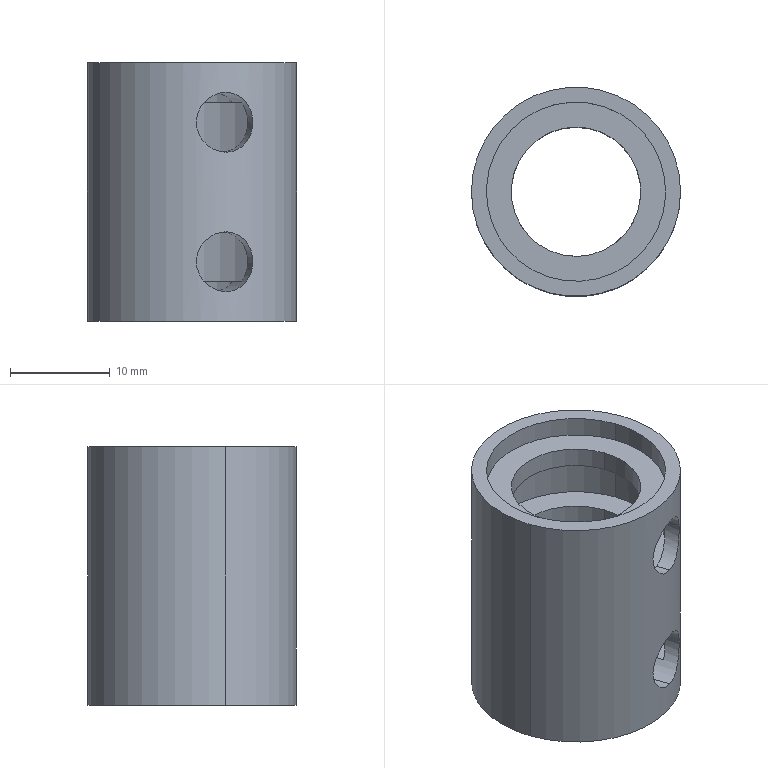Part | SolidWorks | features BaseBody 1 | 1 solid | 30 faces | box 21 x 21 x 26 mm | volume 3749 mm3 | cylinder 22 | plane 8 | commonest cylinder face diameters 18 x10 13 x6 6 x4 21 x2
STEP:
#1=CARTESIAN_POINT('',(25.414,-16.923,-244.5));
#2=VERTEX_POINT('',#1);
#3=CARTESIAN_POINT('',(25.414,-16.923,-250.5));
#4=VERTEX_POINT('',#3);
#5=CARTESIAN_POINT('',(25.414,-16.923,-244.5));
#6=CARTESIAN_POINT('',(25.599,-16.859,-244.5));
#7=CARTESIAN_POINT('',(25.784,-16.79,-244.519));
#8=CARTESIAN_POINT('',(26.145,-16.642,-244.597));
#9=CARTESIAN_POINT('',(26.317,-16.566,-244.654));
#10=CARTESIAN_POINT('',(26.646,-16.411,-244.805));
#11=CARTESIAN_POINT('',(26.804,-16.331,-244.899));
#12=CARTESIAN_POINT('',(27.094,-16.175,-245.116));
#13=CARTESIAN_POINT('',(27.227,-16.1,-245.24));
#14=CARTESIAN_POINT('',(27.47,-15.956,-245.517));
#15=CARTESIAN_POINT('',(27.579,-15.888,-245.67));
#16=CARTESIAN_POINT('',(27.767,-15.767,-245.993));
#17=CARTESIAN_POINT('',(27.846,-15.714,-246.165));
#18=CARTESIAN_POINT('',(27.977,-15.625,-246.531));
#19=CARTESIAN_POINT('',(28.025,-15.591,-246.719));
#20=CARTESIAN_POINT('',(28.091,-15.545,-247.103));
#21=CARTESIAN_POINT('',(28.108,-15.533,-247.302));
#22=CARTESIAN_POINT('',(28.108,-15.532,-247.697));
#23=CARTESIAN_POINT('',(28.091,-15.544,-247.893));
#24=CARTESIAN_POINT('',(28.026,-15.591,-248.279));
#25=CARTESIAN_POINT('',(27.976,-15.625,-248.47));
#26=CARTESIAN_POINT('',(27.783,-15.757,-249.012));
#27=CARTESIAN_POINT('',(27.591,-15.884,-249.345));
#28=CARTESIAN_POINT('',(27.229,-16.099,-249.758));
#29=CARTESIAN_POINT('',(27.094,-16.176,-249.884));
#30=CARTESIAN_POINT('',(26.803,-16.331,-250.102));
#31=CARTESIAN_POINT('',(26.648,-16.41,-250.194));
#32=CARTESIAN_POINT('',(26.32,-16.565,-250.345));
#33=CARTESIAN_POINT('',(26.144,-16.643,-250.403));
#34=CARTESIAN_POINT('',(25.786,-16.789,-250.48));
#35=CARTESIAN_POINT('',(25.602,-16.858,-250.5));
#36=CARTESIAN_POINT('',(25.414,-16.923,-250.5));
#37=B_SPLINE_CURVE_WITH_KNOTS('',3,(#5,#6,#7,#8,#9,#10,#11,#12,#13,#14,#15,#16,#17,#18,#19,#20,#21,#22,#23,#24,#25,#26,#27,#28,#29,#30,#31,#32,#33,#34,#35,#36),.UNSPECIFIED.,.F.,.F.,(4,2,2,2,2,2,2,2,2,2,2,2,2,2,2,4),(0.009429,0.01002,0.01061,0.0112,0.01179,0.01237,0.01296,0.01355,0.01414,0.01473,0.01532,0.0165,0.01709,0.01768,0.01827,0.01885),.UNSPECIFIED.);
#38=EDGE_CURVE('',#2,#4,#37,.T.);
#39=ORIENTED_EDGE('',*,*,#38,.F.);
#40=CARTESIAN_POINT('',(24.925,-15.505,-244.5));
#41=VERTEX_POINT('',#40);
#42=CARTESIAN_POINT('',(29.483,-28.742,-244.5));
#43=DIRECTION('',(-0.3256,0.9455,0.));
#44=VECTOR('',#43,1000.);
#45=LINE('',#42,#44);
#46=EDGE_CURVE('',#2,#41,#45,.T.);
#47=ORIENTED_EDGE('',*,*,#46,.T.);
#48=CARTESIAN_POINT('',(26.948,-14.51,-249.5));
#49=VERTEX_POINT('',#48);
#50=CARTESIAN_POINT('',(26.948,-14.51,-249.5));
#51=CARTESIAN_POINT('',(27.113,-14.401,-249.285));
#52=CARTESIAN_POINT('',(27.247,-14.305,-249.048));
#53=CARTESIAN_POINT('',(27.403,-14.189,-248.658));
#54=CARTESIAN_POINT('',(27.448,-14.156,-248.523));
#55=CARTESIAN_POINT('',(27.518,-14.101,-248.248));
#56=CARTESIAN_POINT('',(27.545,-14.08,-248.108));
#57=CARTESIAN_POINT('',(27.583,-14.051,-247.823));
#58=CARTESIAN_POINT('',(27.593,-14.042,-247.677));
#59=CARTESIAN_POINT('',(27.595,-14.04,-247.386));
#60=CARTESIAN_POINT('',(27.588,-14.046,-247.242));
#61=CARTESIAN_POINT('',(27.54,-14.084,-246.814));
#62=CARTESIAN_POINT('',(27.473,-14.138,-246.531));
#63=CARTESIAN_POINT('',(27.275,-14.285,-246.009));
#64=CARTESIAN_POINT('',(27.142,-14.381,-245.763));
#65=CARTESIAN_POINT('',(26.903,-14.54,-245.439));
#66=CARTESIAN_POINT('',(26.816,-14.596,-245.337));
#67=CARTESIAN_POINT('',(26.629,-14.711,-245.149));
#68=CARTESIAN_POINT('',(26.527,-14.772,-245.061));
#69=CARTESIAN_POINT('',(26.209,-14.952,-244.828));
#70=CARTESIAN_POINT('',(25.974,-15.073,-244.707));
#71=CARTESIAN_POINT('',(25.465,-15.304,-244.542));
#72=CARTESIAN_POINT('',(25.201,-15.41,-244.5));
#73=CARTESIAN_POINT('',(24.925,-15.505,-244.5));
#74=B_SPLINE_CURVE_WITH_KNOTS('',3,(#50,#51,#52,#53,#54,#55,#56,#57,#58,#59,#60,#61,#62,#63,#64,#65,#66,#67,#68,#69,#70,#71,#72,#73),.UNSPECIFIED.,.F.,.F.,(4,2,2,2,2,2,2,2,2,2,2,4),(0.,0.0008651,0.001298,0.00173,0.002163,0.002595,0.00346,0.004325,0.004758,0.00519,0.006055,0.00692),.UNSPECIFIED.);
#75=EDGE_CURVE('',#49,#41,#74,.T.);
#76=ORIENTED_EDGE('',*,*,#75,.F.);
#77=CARTESIAN_POINT('',(26.096,-12.038,-249.5));
#78=VERTEX_POINT('',#77);
#79=CARTESIAN_POINT('',(31.598,-28.014,-249.5));
#80=DIRECTION('',(0.3256,-0.9455,0.));
#81=VECTOR('',#80,1000.);
#82=LINE('',#79,#81);
#83=EDGE_CURVE('',#78,#49,#82,.T.);
#84=ORIENTED_EDGE('',*,*,#83,.F.);
#85=CARTESIAN_POINT('',(24.111,-13.141,-250.5));
#86=VERTEX_POINT('',#85);
#87=CARTESIAN_POINT('',(24.111,-13.141,-250.5));
#88=CARTESIAN_POINT('',(24.312,-13.072,-250.5));
#89=CARTESIAN_POINT('',(24.511,-12.992,-250.477));
#90=CARTESIAN_POINT('',(24.891,-12.818,-250.387));
#91=CARTESIAN_POINT('',(25.07,-12.725,-250.321));
#92=CARTESIAN_POINT('',(25.409,-12.53,-250.148));
#93=CARTESIAN_POINT('',(25.567,-12.429,-250.041));
#94=CARTESIAN_POINT('',(25.852,-12.23,-249.796));
#95=CARTESIAN_POINT('',(25.981,-12.131,-249.656));
#96=CARTESIAN_POINT('',(26.096,-12.038,-249.5));
#97=B_SPLINE_CURVE_WITH_KNOTS('',3,(#87,#88,#89,#90,#91,#92,#93,#94,#95,#96),.UNSPECIFIED.,.F.,.F.,(4,2,2,2,4),(0.002551,0.003187,0.003823,0.00446,0.005096),.UNSPECIFIED.);
#98=EDGE_CURVE('',#86,#78,#97,.T.);
#99=ORIENTED_EDGE('',*,*,#98,.F.);
#100=CARTESIAN_POINT('',(29.483,-28.742,-250.5));
#101=DIRECTION('',(-0.3256,0.9455,0.));
#102=VECTOR('',#101,1000.);
#103=LINE('',#100,#102);
#104=EDGE_CURVE('',#4,#86,#103,.T.);
#105=ORIENTED_EDGE('',*,*,#104,.F.);
#106=EDGE_LOOP('',(#39,#47,#76,#84,#99,#105));
#107=FACE_OUTER_BOUND('',#106,.T.);
#108=CARTESIAN_POINT('',(29.483,-28.742,-247.5));
#109=DIRECTION('',(-0.3256,0.9455,0.));
#110=DIRECTION('',(0.,0.,-1.));
#111=AXIS2_PLACEMENT_3D('',#108,#109,#110);
#112=CYLINDRICAL_SURFACE('',#111,3.);
#113=ADVANCED_FACE('',(#107),#112,.F.);
#114=CARTESIAN_POINT('',(25.414,-16.923,-230.5));
#115=VERTEX_POINT('',#114);
#116=CARTESIAN_POINT('',(25.414,-16.923,-236.5));
#117=VERTEX_POINT('',#116);
#118=CARTESIAN_POINT('',(25.414,-16.923,-230.5));
#119=CARTESIAN_POINT('',(25.599,-16.859,-230.5));
#120=CARTESIAN_POINT('',(25.784,-16.79,-230.519));
#121=CARTESIAN_POINT('',(26.145,-16.642,-230.597));
#122=CARTESIAN_POINT('',(26.317,-16.566,-230.654));
#123=CARTESIAN_POINT('',(26.646,-16.411,-230.805));
#124=CARTESIAN_POINT('',(26.804,-16.331,-230.899));
#125=CARTESIAN_POINT('',(27.094,-16.175,-231.116));
#126=CARTESIAN_POINT('',(27.227,-16.1,-231.24));
#127=CARTESIAN_POINT('',(27.47,-15.956,-231.517));
#128=CARTESIAN_POINT('',(27.579,-15.888,-231.67));
#129=CARTESIAN_POINT('',(27.767,-15.767,-231.993));
#130=CARTESIAN_POINT('',(27.846,-15.714,-232.165));
#131=CARTESIAN_POINT('',(27.977,-15.625,-232.531));
#132=CARTESIAN_POINT('',(28.025,-15.591,-232.719));
#133=CARTESIAN_POINT('',(28.091,-15.545,-233.103));
#134=CARTESIAN_POINT('',(28.108,-15.533,-233.302));
#135=CARTESIAN_POINT('',(28.108,-15.532,-233.697));
#136=CARTESIAN_POINT('',(28.091,-15.544,-233.893));
#137=CARTESIAN_POINT('',(28.026,-15.591,-234.279));
#138=CARTESIAN_POINT('',(27.976,-15.625,-234.47));
#139=CARTESIAN_POINT('',(27.783,-15.757,-235.012));
#140=CARTESIAN_POINT('',(27.591,-15.884,-235.345));
#141=CARTESIAN_POINT('',(27.229,-16.099,-235.758));
#142=CARTESIAN_POINT('',(27.094,-16.176,-235.884));
#143=CARTESIAN_POINT('',(26.803,-16.331,-236.102));
#144=CARTESIAN_POINT('',(26.648,-16.41,-236.194));
#145=CARTESIAN_POINT('',(26.32,-16.565,-236.345));
#146=CARTESIAN_POINT('',(26.144,-16.643,-236.403));
#147=CARTESIAN_POINT('',(25.786,-16.789,-236.48));
#148=CARTESIAN_POINT('',(25.602,-16.858,-236.5));
#149=CARTESIAN_POINT('',(25.414,-16.923,-236.5));
#150=B_SPLINE_CURVE_WITH_KNOTS('',3,(#118,#119,#120,#121,#122,#123,#124,#125,#126,#127,#128,#129,#130,#131,#132,#133,#134,#135,#136,#137,#138,#139,#140,#141,#142,#143,#144,#145,#146,#147,#148,#149),.UNSPECIFIED.,.F.,.F.,(4,2,2,2,2,2,2,2,2,2,2,2,2,2,2,4),(0.009429,0.01002,0.01061,0.0112,0.01179,0.01237,0.01296,0.01355,0.01414,0.01473,0.01532,0.0165,0.01709,0.01768,0.01827,0.01885),.UNSPECIFIED.);
#151=EDGE_CURVE('',#115,#117,#150,.T.);
#152=ORIENTED_EDGE('',*,*,#151,.F.);
#153=CARTESIAN_POINT('',(24.111,-13.141,-230.5));
#154=VERTEX_POINT('',#153);
#155=CARTESIAN_POINT('',(29.483,-28.742,-230.5));
#156=DIRECTION('',(-0.3256,0.9455,0.));
#157=VECTOR('',#156,1000.);
#158=LINE('',#155,#157);
#159=EDGE_CURVE('',#115,#154,#158,.T.);
#160=ORIENTED_EDGE('',*,*,#159,.T.);
#161=CARTESIAN_POINT('',(26.096,-12.038,-231.5));
#162=VERTEX_POINT('',#161);
#163=CARTESIAN_POINT('',(26.096,-12.038,-231.5));
#164=CARTESIAN_POINT('',(25.981,-12.132,-231.344));
#165=CARTESIAN_POINT('',(25.853,-12.229,-231.205));
#166=CARTESIAN_POINT('',(25.568,-12.428,-230.96));
#167=CARTESIAN_POINT('',(25.409,-12.53,-230.852));
#168=CARTESIAN_POINT('',(25.071,-12.725,-230.679));
#169=CARTESIAN_POINT('',(24.892,-12.818,-230.613));
#170=CARTESIAN_POINT('',(24.512,-12.992,-230.523));
#171=CARTESIAN_POINT('',(24.312,-13.072,-230.5));
#172=CARTESIAN_POINT('',(24.111,-13.141,-230.5));
#173=B_SPLINE_CURVE_WITH_KNOTS('',3,(#163,#164,#165,#166,#167,#168,#169,#170,#171,#172),.UNSPECIFIED.,.F.,.F.,(4,2,2,2,4),(0.,0.0006377,0.001275,0.001913,0.002551),.UNSPECIFIED.);
#174=EDGE_CURVE('',#162,#154,#173,.T.);
#175=ORIENTED_EDGE('',*,*,#174,.F.);
#176=CARTESIAN_POINT('',(26.948,-14.51,-231.5));
#177=VERTEX_POINT('',#176);
#178=CARTESIAN_POINT('',(31.598,-28.014,-231.5));
#179=DIRECTION('',(-0.3256,0.9455,0.));
#180=VECTOR('',#179,1000.);
#181=LINE('',#178,#180);
#182=EDGE_CURVE('',#177,#162,#181,.T.);
#183=ORIENTED_EDGE('',*,*,#182,.F.);
#184=CARTESIAN_POINT('',(24.925,-15.505,-236.5));
#185=VERTEX_POINT('',#184);
#186=CARTESIAN_POINT('',(24.925,-15.505,-236.5));
#187=CARTESIAN_POINT('',(25.201,-15.41,-236.5));
#188=CARTESIAN_POINT('',(25.468,-15.303,-236.458));
#189=CARTESIAN_POINT('',(25.847,-15.13,-236.334));
#190=CARTESIAN_POINT('',(25.971,-15.07,-236.283));
#191=CARTESIAN_POINT('',(26.205,-14.951,-236.162));
#192=CARTESIAN_POINT('',(26.317,-14.891,-236.093));
#193=CARTESIAN_POINT('',(26.529,-14.771,-235.937));
#194=CARTESIAN_POINT('',(26.63,-14.711,-235.85));
#195=CARTESIAN_POINT('',(26.818,-14.595,-235.661));
#196=CARTESIAN_POINT('',(26.904,-14.539,-235.56));
#197=CARTESIAN_POINT('',(27.143,-14.38,-235.236));
#198=CARTESIAN_POINT('',(27.276,-14.284,-234.99));
#199=CARTESIAN_POINT('',(27.423,-14.174,-234.599));
#200=CARTESIAN_POINT('',(27.464,-14.143,-234.465));
#201=CARTESIAN_POINT('',(27.531,-14.091,-234.187));
#202=CARTESIAN_POINT('',(27.556,-14.072,-234.044));
#203=CARTESIAN_POINT('',(27.588,-14.046,-233.758));
#204=CARTESIAN_POINT('',(27.595,-14.041,-233.614));
#205=CARTESIAN_POINT('',(27.593,-14.042,-233.326));
#206=CARTESIAN_POINT('',(27.583,-14.05,-233.179));
#207=CARTESIAN_POINT('',(27.527,-14.094,-232.75));
#208=CARTESIAN_POINT('',(27.456,-14.15,-232.474));
#209=CARTESIAN_POINT('',(27.247,-14.305,-231.952));
#210=CARTESIAN_POINT('',(27.113,-14.401,-231.715));
#211=CARTESIAN_POINT('',(26.948,-14.51,-231.5));
#212=B_SPLINE_CURVE_WITH_KNOTS('',3,(#186,#187,#188,#189,#190,#191,#192,#193,#194,#195,#196,#197,#198,#199,#200,#201,#202,#203,#204,#205,#206,#207,#208,#209,#210,#211),.UNSPECIFIED.,.F.,.F.,(4,2,2,2,2,2,2,2,2,2,2,2,4),(0.00692,0.007785,0.008217,0.00865,0.009082,0.009514,0.01038,0.01081,0.01124,0.01168,0.01211,0.01297,0.01384),.UNSPECIFIED.);
#213=EDGE_CURVE('',#185,#177,#212,.T.);
#214=ORIENTED_EDGE('',*,*,#213,.F.);
#215=CARTESIAN_POINT('',(29.483,-28.742,-236.5));
#216=DIRECTION('',(-0.3256,0.9455,0.));
#217=VECTOR('',#216,1000.);
#218=LINE('',#215,#217);
#219=EDGE_CURVE('',#117,#185,#218,.T.);
#220=ORIENTED_EDGE('',*,*,#219,.F.);
#221=EDGE_LOOP('',(#152,#160,#175,#183,#214,#220));
#222=FACE_OUTER_BOUND('',#221,.T.);
#223=CARTESIAN_POINT('',(29.483,-28.742,-233.5));
#224=DIRECTION('',(-0.3256,0.9455,0.));
#225=DIRECTION('',(0.,0.,-1.));
#226=AXIS2_PLACEMENT_3D('',#223,#224,#225);
#227=CYLINDRICAL_SURFACE('',#226,3.);
#228=ADVANCED_FACE('',(#222),#227,.F.);
#229=CARTESIAN_POINT('',(30.505,-4.065,-229.5));
#230=VERTEX_POINT('',#229);
#231=CARTESIAN_POINT('',(13.486,-9.925,-229.5));
#232=VERTEX_POINT('',#231);
#233=CARTESIAN_POINT('',(21.995,-6.995,-229.5));
#234=DIRECTION('',(0.,0.,-1.));
#235=DIRECTION('',(0.9455,0.3256,0.));
#236=AXIS2_PLACEMENT_3D('',#233,#234,#235);
#237=CIRCLE('',#236,9.);
#238=EDGE_CURVE('',#230,#232,#237,.T.);
#239=ORIENTED_EDGE('',*,*,#238,.T.);
#240=CARTESIAN_POINT('',(13.486,-9.925,-227.5));
#241=VERTEX_POINT('',#240);
#242=CARTESIAN_POINT('',(13.486,-9.925,-227.5));
#243=DIRECTION('',(0.,0.,1.));
#244=VECTOR('',#243,1000.);
#245=LINE('',#242,#244);
#246=EDGE_CURVE('',#232,#241,#245,.T.);
#247=ORIENTED_EDGE('',*,*,#246,.T.);
#248=CARTESIAN_POINT('',(30.505,-4.065,-227.5));
#249=VERTEX_POINT('',#248);
#250=CARTESIAN_POINT('',(21.995,-6.995,-227.5));
#251=DIRECTION('',(0.,0.,-1.));
#252=DIRECTION('',(0.9455,0.3256,0.));
#253=AXIS2_PLACEMENT_3D('',#250,#251,#252);
#254=CIRCLE('',#253,9.);
#255=EDGE_CURVE('',#249,#241,#254,.T.);
#256=ORIENTED_EDGE('',*,*,#255,.F.);
#257=CARTESIAN_POINT('',(30.505,-4.065,-227.5));
#258=DIRECTION('',(0.,0.,1.));
#259=VECTOR('',#258,1000.);
#260=LINE('',#257,#259);
#261=EDGE_CURVE('',#230,#249,#260,.T.);
#262=ORIENTED_EDGE('',*,*,#261,.F.);
#263=EDGE_LOOP('',(#239,#247,#256,#262));
#264=FACE_OUTER_BOUND('',#263,.T.);
#265=CARTESIAN_POINT('',(21.995,-6.995,-227.5));
#266=DIRECTION('',(0.,0.,1.));
#267=DIRECTION('',(0.9455,0.3256,0.));
#268=AXIS2_PLACEMENT_3D('',#265,#266,#267);
#269=CYLINDRICAL_SURFACE('',#268,9.);
#270=ADVANCED_FACE('',(#264),#269,.F.);
#271=CARTESIAN_POINT('',(30.505,-4.065,-253.5));
#272=VERTEX_POINT('',#271);
#273=CARTESIAN_POINT('',(13.486,-9.925,-253.5));
#274=VERTEX_POINT('',#273);
#275=CARTESIAN_POINT('',(21.995,-6.995,-253.5));
#276=DIRECTION('',(0.,0.,-1.));
#277=DIRECTION('',(0.9455,0.3256,0.));
#278=AXIS2_PLACEMENT_3D('',#275,#276,#277);
#279=CIRCLE('',#278,9.);
#280=EDGE_CURVE('',#272,#274,#279,.T.);
#281=ORIENTED_EDGE('',*,*,#280,.T.);
#282=CARTESIAN_POINT('',(13.486,-9.925,-251.5));
#283=VERTEX_POINT('',#282);
#284=CARTESIAN_POINT('',(13.486,-9.925,-227.5));
#285=DIRECTION('',(0.,0.,1.));
#286=VECTOR('',#285,1000.);
#287=LINE('',#284,#286);
#288=EDGE_CURVE('',#274,#283,#287,.T.);
#289=ORIENTED_EDGE('',*,*,#288,.T.);
#290=CARTESIAN_POINT('',(30.505,-4.065,-251.5));
#291=VERTEX_POINT('',#290);
#292=CARTESIAN_POINT('',(21.995,-6.995,-251.5));
#293=DIRECTION('',(0.,0.,-1.));
#294=DIRECTION('',(0.9455,0.3256,0.));
#295=AXIS2_PLACEMENT_3D('',#292,#293,#294);
#296=CIRCLE('',#295,9.);
#297=EDGE_CURVE('',#291,#283,#296,.T.);
#298=ORIENTED_EDGE('',*,*,#297,.F.);
#299=CARTESIAN_POINT('',(30.505,-4.065,-227.5));
#300=DIRECTION('',(0.,0.,1.));
#301=VECTOR('',#300,1000.);
#302=LINE('',#299,#301);
#303=EDGE_CURVE('',#272,#291,#302,.T.);
#304=ORIENTED_EDGE('',*,*,#303,.F.);
#305=EDGE_LOOP('',(#281,#289,#298,#304));
#306=FACE_OUTER_BOUND('',#305,.T.);
#307=CARTESIAN_POINT('',(21.995,-6.995,-227.5));
#308=DIRECTION('',(0.,0.,1.));
#309=DIRECTION('',(0.9455,0.3256,0.));
#310=AXIS2_PLACEMENT_3D('',#307,#308,#309);
#311=CYLINDRICAL_SURFACE('',#310,9.);
#312=ADVANCED_FACE('',(#306),#311,.F.);
#313=CARTESIAN_POINT('',(28.141,-4.879,-244.5));
#314=VERTEX_POINT('',#313);
#315=CARTESIAN_POINT('',(15.849,-9.111,-244.5));
#316=VERTEX_POINT('',#315);
#317=CARTESIAN_POINT('',(21.995,-6.995,-244.5));
#318=DIRECTION('',(0.,0.,-1.));
#319=DIRECTION('',(0.9455,0.3256,0.));
#320=AXIS2_PLACEMENT_3D('',#317,#318,#319);
#321=CIRCLE('',#320,6.5);
#322=EDGE_CURVE('',#314,#316,#321,.T.);
#323=ORIENTED_EDGE('',*,*,#322,.T.);
#324=CARTESIAN_POINT('',(15.849,-9.111,-236.5));
#325=VERTEX_POINT('',#324);
#326=CARTESIAN_POINT('',(15.849,-9.111,-227.5));
#327=DIRECTION('',(0.,0.,1.));
#328=VECTOR('',#327,1000.);
#329=LINE('',#326,#328);
#330=EDGE_CURVE('',#316,#325,#329,.T.);
#331=ORIENTED_EDGE('',*,*,#330,.T.);
#332=CARTESIAN_POINT('',(28.141,-4.879,-236.5));
#333=VERTEX_POINT('',#332);
#334=CARTESIAN_POINT('',(21.995,-6.995,-236.5));
#335=DIRECTION('',(0.,0.,-1.));
#336=DIRECTION('',(0.9455,0.3256,0.));
#337=AXIS2_PLACEMENT_3D('',#334,#335,#336);
#338=CIRCLE('',#337,6.5);
#339=EDGE_CURVE('',#333,#325,#338,.T.);
#340=ORIENTED_EDGE('',*,*,#339,.F.);
#341=CARTESIAN_POINT('',(28.141,-4.879,-227.5));
#342=DIRECTION('',(0.,0.,1.));
#343=VECTOR('',#342,1000.);
#344=LINE('',#341,#343);
#345=EDGE_CURVE('',#314,#333,#344,.T.);
#346=ORIENTED_EDGE('',*,*,#345,.F.);
#347=EDGE_LOOP('',(#323,#331,#340,#346));
#348=FACE_OUTER_BOUND('',#347,.T.);
#349=CARTESIAN_POINT('',(21.995,-6.995,-227.5));
#350=DIRECTION('',(0.,0.,1.));
#351=DIRECTION('',(0.9455,0.3256,0.));
#352=AXIS2_PLACEMENT_3D('',#349,#350,#351);
#353=CYLINDRICAL_SURFACE('',#352,6.5);
#354=ADVANCED_FACE('',(#348),#353,.F.);
#355=CARTESIAN_POINT('',(13.486,-9.925,-236.5));
#356=VERTEX_POINT('',#355);
#357=CARTESIAN_POINT('',(21.995,-6.995,-236.5));
#358=DIRECTION('',(0.,0.,-1.));
#359=DIRECTION('',(0.9455,0.3256,0.));
#360=AXIS2_PLACEMENT_3D('',#357,#358,#359);
#361=CIRCLE('',#360,9.);
#362=EDGE_CURVE('',#185,#356,#361,.T.);
#363=ORIENTED_EDGE('',*,*,#362,.T.);
#364=CARTESIAN_POINT('',(13.486,-9.925,-231.5));
#365=VERTEX_POINT('',#364);
#366=CARTESIAN_POINT('',(13.486,-9.925,-227.5));
#367=DIRECTION('',(0.,0.,1.));
#368=VECTOR('',#367,1000.);
#369=LINE('',#366,#368);
#370=EDGE_CURVE('',#356,#365,#369,.T.);
#371=ORIENTED_EDGE('',*,*,#370,.T.);
#372=CARTESIAN_POINT('',(22.719,-15.966,-231.5));
#373=VERTEX_POINT('',#372);
#374=CARTESIAN_POINT('',(21.995,-6.995,-231.5));
#375=DIRECTION('',(0.,0.,-1.));
#376=DIRECTION('',(0.9455,0.3256,0.));
#377=AXIS2_PLACEMENT_3D('',#374,#375,#376);
#378=CIRCLE('',#377,9.);
#379=EDGE_CURVE('',#373,#365,#378,.T.);
#380=ORIENTED_EDGE('',*,*,#379,.F.);
#381=CARTESIAN_POINT('',(22.719,-15.966,-231.5));
#382=CARTESIAN_POINT('',(22.522,-15.982,-231.715));
#383=CARTESIAN_POINT('',(22.357,-15.989,-231.952));
#384=CARTESIAN_POINT('',(22.163,-15.994,-232.342));
#385=CARTESIAN_POINT('',(22.107,-15.995,-232.477));
#386=CARTESIAN_POINT('',(22.018,-15.995,-232.752));
#387=CARTESIAN_POINT('',(21.983,-15.995,-232.892));
#388=CARTESIAN_POINT('',(21.936,-15.995,-233.177));
#389=CARTESIAN_POINT('',(21.923,-15.995,-233.323));
#390=CARTESIAN_POINT('',(21.92,-15.995,-233.614));
#391=CARTESIAN_POINT('',(21.929,-15.995,-233.758));
#392=CARTESIAN_POINT('',(21.99,-15.995,-234.186));
#393=CARTESIAN_POINT('',(22.076,-15.996,-234.469));
#394=CARTESIAN_POINT('',(22.323,-15.99,-234.991));
#395=CARTESIAN_POINT('',(22.486,-15.984,-235.237));
#396=CARTESIAN_POINT('',(22.773,-15.962,-235.561));
#397=CARTESIAN_POINT('',(22.875,-15.953,-235.663));
#398=CARTESIAN_POINT('',(23.095,-15.928,-235.851));
#399=CARTESIAN_POINT('',(23.212,-15.913,-235.939));
#400=CARTESIAN_POINT('',(23.573,-15.859,-236.172));
#401=CARTESIAN_POINT('',(23.833,-15.81,-236.293));
#402=CARTESIAN_POINT('',(24.376,-15.679,-236.458));
#403=CARTESIAN_POINT('',(24.65,-15.6,-236.5));
#404=CARTESIAN_POINT('',(24.925,-15.505,-236.5));
#405=B_SPLINE_CURVE_WITH_KNOTS('',3,(#381,#382,#383,#384,#385,#386,#387,#388,#389,#390,#391,#392,#393,#394,#395,#396,#397,#398,#399,#400,#401,#402,#403,#404),.UNSPECIFIED.,.F.,.F.,(4,2,2,2,2,2,2,2,2,2,2,4),(0.,0.0008651,0.001298,0.00173,0.002163,0.002595,0.00346,0.004325,0.004758,0.00519,0.006055,0.00692),.UNSPECIFIED.);
#406=EDGE_CURVE('',#373,#185,#405,.T.);
#407=ORIENTED_EDGE('',*,*,#406,.T.);
#408=EDGE_LOOP('',(#363,#371,#380,#407));
#409=FACE_OUTER_BOUND('',#408,.T.);
#410=CARTESIAN_POINT('',(21.995,-6.995,-227.5));
#411=DIRECTION('',(0.,0.,1.));
#412=DIRECTION('',(0.9455,0.3256,0.));
#413=AXIS2_PLACEMENT_3D('',#410,#411,#412);
#414=CYLINDRICAL_SURFACE('',#413,9.);
#415=ADVANCED_FACE('',(#409),#414,.F.);
#416=ORIENTED_EDGE('',*,*,#370,.F.);
#417=CARTESIAN_POINT('',(30.505,-4.065,-236.5));
#418=VERTEX_POINT('',#417);
#419=CARTESIAN_POINT('',(21.995,-6.995,-236.5));
#420=DIRECTION('',(0.,0.,-1.));
#421=DIRECTION('',(0.9455,0.3256,0.));
#422=AXIS2_PLACEMENT_3D('',#419,#420,#421);
#423=CIRCLE('',#422,9.);
#424=EDGE_CURVE('',#356,#418,#423,.T.);
#425=ORIENTED_EDGE('',*,*,#424,.T.);
#426=CARTESIAN_POINT('',(30.505,-4.065,-231.5));
#427=VERTEX_POINT('',#426);
#428=CARTESIAN_POINT('',(30.505,-4.065,-227.5));
#429=DIRECTION('',(0.,0.,1.));
#430=VECTOR('',#429,1000.);
#431=LINE('',#428,#430);
#432=EDGE_CURVE('',#418,#427,#431,.T.);
#433=ORIENTED_EDGE('',*,*,#432,.T.);
#434=CARTESIAN_POINT('',(21.995,-6.995,-231.5));
#435=DIRECTION('',(0.,0.,-1.));
#436=DIRECTION('',(0.9455,0.3256,0.));
#437=AXIS2_PLACEMENT_3D('',#434,#435,#436);
#438=CIRCLE('',#437,9.);
#439=EDGE_CURVE('',#365,#427,#438,.T.);
#440=ORIENTED_EDGE('',*,*,#439,.F.);
#441=EDGE_LOOP('',(#416,#425,#433,#440));
#442=FACE_OUTER_BOUND('',#441,.T.);
#443=CARTESIAN_POINT('',(21.995,-6.995,-227.5));
#444=DIRECTION('',(0.,0.,1.));
#445=DIRECTION('',(0.9455,0.3256,0.));
#446=AXIS2_PLACEMENT_3D('',#443,#444,#445);
#447=CYLINDRICAL_SURFACE('',#446,9.);
#448=ADVANCED_FACE('',(#442),#447,.F.);
#449=CARTESIAN_POINT('',(21.868,-13.494,-231.5));
#450=VERTEX_POINT('',#449);
#451=CARTESIAN_POINT('',(15.849,-9.111,-231.5));
#452=VERTEX_POINT('',#451);
#453=CARTESIAN_POINT('',(21.995,-6.995,-231.5));
#454=DIRECTION('',(0.,0.,-1.));
#455=DIRECTION('',(0.9455,0.3256,0.));
#456=AXIS2_PLACEMENT_3D('',#453,#454,#455);
#457=CIRCLE('',#456,6.5);
#458=EDGE_CURVE('',#450,#452,#457,.T.);
#459=ORIENTED_EDGE('',*,*,#458,.T.);
#460=CARTESIAN_POINT('',(15.849,-9.111,-229.5));
#461=VERTEX_POINT('',#460);
#462=CARTESIAN_POINT('',(15.849,-9.111,-227.5));
#463=DIRECTION('',(0.,0.,1.));
#464=VECTOR('',#463,1000.);
#465=LINE('',#462,#464);
#466=EDGE_CURVE('',#452,#461,#465,.T.);
#467=ORIENTED_EDGE('',*,*,#466,.T.);
#468=CARTESIAN_POINT('',(28.141,-4.879,-229.5));
#469=VERTEX_POINT('',#468);
#470=CARTESIAN_POINT('',(21.995,-6.995,-229.5));
#471=DIRECTION('',(0.,0.,-1.));
#472=DIRECTION('',(0.9455,0.3256,0.));
#473=AXIS2_PLACEMENT_3D('',#470,#471,#472);
#474=CIRCLE('',#473,6.5);
#475=EDGE_CURVE('',#469,#461,#474,.T.);
#476=ORIENTED_EDGE('',*,*,#475,.F.);
#477=CARTESIAN_POINT('',(28.141,-4.879,-231.5));
#478=VERTEX_POINT('',#477);
#479=CARTESIAN_POINT('',(28.141,-4.879,-227.5));
#480=DIRECTION('',(0.,0.,1.));
#481=VECTOR('',#480,1000.);
#482=LINE('',#479,#481);
#483=EDGE_CURVE('',#478,#469,#482,.T.);
#484=ORIENTED_EDGE('',*,*,#483,.F.);
#485=CARTESIAN_POINT('',(21.995,-6.995,-231.5));
#486=DIRECTION('',(0.,0.,-1.));
#487=DIRECTION('',(0.9455,0.3256,0.));
#488=AXIS2_PLACEMENT_3D('',#485,#486,#487);
#489=CIRCLE('',#488,6.5);
#490=EDGE_CURVE('',#478,#162,#489,.T.);
#491=ORIENTED_EDGE('',*,*,#490,.T.);
#492=ORIENTED_EDGE('',*,*,#174,.T.);
#493=CARTESIAN_POINT('',(24.111,-13.141,-230.5));
#494=CARTESIAN_POINT('',(23.911,-13.21,-230.5));
#495=CARTESIAN_POINT('',(23.705,-13.27,-230.523));
#496=CARTESIAN_POINT('',(23.298,-13.367,-230.613));
#497=CARTESIAN_POINT('',(23.1,-13.404,-230.679));
#498=CARTESIAN_POINT('',(22.713,-13.458,-230.852));
#499=CARTESIAN_POINT('',(22.526,-13.476,-230.959));
#500=CARTESIAN_POINT('',(22.179,-13.495,-231.204));
#501=CARTESIAN_POINT('',(22.016,-13.497,-231.344));
#502=CARTESIAN_POINT('',(21.868,-13.494,-231.5));
#503=B_SPLINE_CURVE_WITH_KNOTS('',3,(#493,#494,#495,#496,#497,#498,#499,#500,#501,#502),.UNSPECIFIED.,.F.,.F.,(4,2,2,2,4),(0.002551,0.003187,0.003823,0.00446,0.005096),.UNSPECIFIED.);
#504=EDGE_CURVE('',#154,#450,#503,.T.);
#505=ORIENTED_EDGE('',*,*,#504,.T.);
#506=EDGE_LOOP('',(#459,#467,#476,#484,#491,#492,#505));
#507=FACE_OUTER_BOUND('',#506,.T.);
#508=CARTESIAN_POINT('',(21.995,-6.995,-227.5));
#509=DIRECTION('',(0.,0.,1.));
#510=DIRECTION('',(0.9455,0.3256,0.));
#511=AXIS2_PLACEMENT_3D('',#508,#509,#510);
#512=CYLINDRICAL_SURFACE('',#511,6.5);
#513=ADVANCED_FACE('',(#507),#512,.F.);
#514=CARTESIAN_POINT('',(28.141,-4.879,-251.5));
#515=VERTEX_POINT('',#514);
#516=CARTESIAN_POINT('',(15.849,-9.111,-251.5));
#517=VERTEX_POINT('',#516);
#518=CARTESIAN_POINT('',(21.995,-6.995,-251.5));
#519=DIRECTION('',(0.,0.,-1.));
#520=DIRECTION('',(0.9455,0.3256,0.));
#521=AXIS2_PLACEMENT_3D('',#518,#519,#520);
#522=CIRCLE('',#521,6.5);
#523=EDGE_CURVE('',#515,#517,#522,.T.);
#524=ORIENTED_EDGE('',*,*,#523,.T.);
#525=CARTESIAN_POINT('',(15.849,-9.111,-249.5));
#526=VERTEX_POINT('',#525);
#527=CARTESIAN_POINT('',(15.849,-9.111,-227.5));
#528=DIRECTION('',(0.,0.,1.));
#529=VECTOR('',#528,1000.);
#530=LINE('',#527,#529);
#531=EDGE_CURVE('',#517,#526,#530,.T.);
#532=ORIENTED_EDGE('',*,*,#531,.T.);
#533=CARTESIAN_POINT('',(21.868,-13.494,-249.5));
#534=VERTEX_POINT('',#533);
#535=CARTESIAN_POINT('',(21.995,-6.995,-249.5));
#536=DIRECTION('',(0.,0.,-1.));
#537=DIRECTION('',(0.9455,0.3256,0.));
#538=AXIS2_PLACEMENT_3D('',#535,#536,#537);
#539=CIRCLE('',#538,6.5);
#540=EDGE_CURVE('',#534,#526,#539,.T.);
#541=ORIENTED_EDGE('',*,*,#540,.F.);
#542=CARTESIAN_POINT('',(21.868,-13.494,-249.5));
#543=CARTESIAN_POINT('',(22.017,-13.497,-249.656));
#544=CARTESIAN_POINT('',(22.178,-13.495,-249.795));
#545=CARTESIAN_POINT('',(22.525,-13.476,-250.04));
#546=CARTESIAN_POINT('',(22.713,-13.458,-250.148));
#547=CARTESIAN_POINT('',(23.099,-13.404,-250.321));
#548=CARTESIAN_POINT('',(23.297,-13.367,-250.387));
#549=CARTESIAN_POINT('',(23.704,-13.27,-250.477));
#550=CARTESIAN_POINT('',(23.911,-13.21,-250.5));
#551=CARTESIAN_POINT('',(24.111,-13.141,-250.5));
#552=B_SPLINE_CURVE_WITH_KNOTS('',3,(#542,#543,#544,#545,#546,#547,#548,#549,#550,#551),.UNSPECIFIED.,.F.,.F.,(4,2,2,2,4),(0.,0.0006377,0.001275,0.001913,0.002551),.UNSPECIFIED.);
#553=EDGE_CURVE('',#534,#86,#552,.T.);
#554=ORIENTED_EDGE('',*,*,#553,.T.);
#555=ORIENTED_EDGE('',*,*,#98,.T.);
#556=CARTESIAN_POINT('',(28.141,-4.879,-249.5));
#557=VERTEX_POINT('',#556);
#558=CARTESIAN_POINT('',(21.995,-6.995,-249.5));
#559=DIRECTION('',(0.,0.,-1.));
#560=DIRECTION('',(0.9455,0.3256,0.));
#561=AXIS2_PLACEMENT_3D('',#558,#559,#560);
#562=CIRCLE('',#561,6.5);
#563=EDGE_CURVE('',#557,#78,#562,.T.);
#564=ORIENTED_EDGE('',*,*,#563,.F.);
#565=CARTESIAN_POINT('',(28.141,-4.879,-227.5));
#566=DIRECTION('',(0.,0.,1.));
#567=VECTOR('',#566,1000.);
#568=LINE('',#565,#567);
#569=EDGE_CURVE('',#515,#557,#568,.T.);
#570=ORIENTED_EDGE('',*,*,#569,.F.);
#571=EDGE_LOOP('',(#524,#532,#541,#554,#555,#564,#570));
#572=FACE_OUTER_BOUND('',#571,.T.);
#573=CARTESIAN_POINT('',(21.995,-6.995,-227.5));
#574=DIRECTION('',(0.,0.,1.));
#575=DIRECTION('',(0.9455,0.3256,0.));
#576=AXIS2_PLACEMENT_3D('',#573,#574,#575);
#577=CYLINDRICAL_SURFACE('',#576,6.5);
#578=ADVANCED_FACE('',(#572),#577,.F.);
#579=CARTESIAN_POINT('',(22.719,-15.966,-249.5));
#580=VERTEX_POINT('',#579);
#581=CARTESIAN_POINT('',(13.486,-9.925,-249.5));
#582=VERTEX_POINT('',#581);
#583=CARTESIAN_POINT('',(21.995,-6.995,-249.5));
#584=DIRECTION('',(0.,0.,-1.));
#585=DIRECTION('',(0.9455,0.3256,0.));
#586=AXIS2_PLACEMENT_3D('',#583,#584,#585);
#587=CIRCLE('',#586,9.);
#588=EDGE_CURVE('',#580,#582,#587,.T.);
#589=ORIENTED_EDGE('',*,*,#588,.T.);
#590=CARTESIAN_POINT('',(13.486,-9.925,-244.5));
#591=VERTEX_POINT('',#590);
#592=CARTESIAN_POINT('',(13.486,-9.925,-227.5));
#593=DIRECTION('',(0.,0.,1.));
#594=VECTOR('',#593,1000.);
#595=LINE('',#592,#594);
#596=EDGE_CURVE('',#582,#591,#595,.T.);
#597=ORIENTED_EDGE('',*,*,#596,.T.);
#598=CARTESIAN_POINT('',(21.995,-6.995,-244.5));
#599=DIRECTION('',(0.,0.,-1.));
#600=DIRECTION('',(0.9455,0.3256,0.));
#601=AXIS2_PLACEMENT_3D('',#598,#599,#600);
#602=CIRCLE('',#601,9.);
#603=EDGE_CURVE('',#41,#591,#602,.T.);
#604=ORIENTED_EDGE('',*,*,#603,.F.);
#605=CARTESIAN_POINT('',(24.925,-15.505,-244.5));
#606=CARTESIAN_POINT('',(24.65,-15.6,-244.5));
#607=CARTESIAN_POINT('',(24.374,-15.68,-244.542));
#608=CARTESIAN_POINT('',(23.968,-15.777,-244.666));
#609=CARTESIAN_POINT('',(23.834,-15.806,-244.717));
#610=CARTESIAN_POINT('',(23.576,-15.856,-244.838));
#611=CARTESIAN_POINT('',(23.451,-15.877,-244.907));
#612=CARTESIAN_POINT('',(23.21,-15.914,-245.063));
#613=CARTESIAN_POINT('',(23.093,-15.929,-245.15));
#614=CARTESIAN_POINT('',(22.874,-15.953,-245.339));
#615=CARTESIAN_POINT('',(22.771,-15.962,-245.44));
#616=CARTESIAN_POINT('',(22.485,-15.984,-245.764));
#617=CARTESIAN_POINT('',(22.322,-15.99,-246.01));
#618=CARTESIAN_POINT('',(22.138,-15.994,-246.401));
#619=CARTESIAN_POINT('',(22.086,-15.995,-246.535));
#620=CARTESIAN_POINT('',(22.002,-15.995,-246.813));
#621=CARTESIAN_POINT('',(21.97,-15.995,-246.956));
#622=CARTESIAN_POINT('',(21.929,-15.995,-247.242));
#623=CARTESIAN_POINT('',(21.92,-15.995,-247.386));
#624=CARTESIAN_POINT('',(21.923,-15.995,-247.674));
#625=CARTESIAN_POINT('',(21.936,-15.995,-247.821));
#626=CARTESIAN_POINT('',(22.007,-15.995,-248.25));
#627=CARTESIAN_POINT('',(22.097,-15.995,-248.526));
#628=CARTESIAN_POINT('',(22.357,-15.989,-249.048));
#629=CARTESIAN_POINT('',(22.522,-15.982,-249.285));
#630=CARTESIAN_POINT('',(22.719,-15.966,-249.5));
#631=B_SPLINE_CURVE_WITH_KNOTS('',3,(#605,#606,#607,#608,#609,#610,#611,#612,#613,#614,#615,#616,#617,#618,#619,#620,#621,#622,#623,#624,#625,#626,#627,#628,#629,#630),.UNSPECIFIED.,.F.,.F.,(4,2,2,2,2,2,2,2,2,2,2,2,4),(0.00692,0.007785,0.008217,0.00865,0.009082,0.009514,0.01038,0.01081,0.01124,0.01168,0.01211,0.01297,0.01384),.UNSPECIFIED.);
#632=EDGE_CURVE('',#41,#580,#631,.T.);
#633=ORIENTED_EDGE('',*,*,#632,.T.);
#634=EDGE_LOOP('',(#589,#597,#604,#633));
#635=FACE_OUTER_BOUND('',#634,.T.);
#636=CARTESIAN_POINT('',(21.995,-6.995,-227.5));
#637=DIRECTION('',(0.,0.,1.));
#638=DIRECTION('',(0.9455,0.3256,0.));
#639=AXIS2_PLACEMENT_3D('',#636,#637,#638);
#640=CYLINDRICAL_SURFACE('',#639,9.);
#641=ADVANCED_FACE('',(#635),#640,.F.);
#642=ORIENTED_EDGE('',*,*,#596,.F.);
#643=CARTESIAN_POINT('',(30.505,-4.065,-249.5));
#644=VERTEX_POINT('',#643);
#645=CARTESIAN_POINT('',(21.995,-6.995,-249.5));
#646=DIRECTION('',(0.,0.,-1.));
#647=DIRECTION('',(0.9455,0.3256,0.));
#648=AXIS2_PLACEMENT_3D('',#645,#646,#647);
#649=CIRCLE('',#648,9.);
#650=EDGE_CURVE('',#582,#644,#649,.T.);
#651=ORIENTED_EDGE('',*,*,#650,.T.);
#652=CARTESIAN_POINT('',(30.505,-4.065,-244.5));
#653=VERTEX_POINT('',#652);
#654=CARTESIAN_POINT('',(30.505,-4.065,-227.5));
#655=DIRECTION('',(0.,0.,1.));
#656=VECTOR('',#655,1000.);
#657=LINE('',#654,#656);
#658=EDGE_CURVE('',#644,#653,#657,.T.);
#659=ORIENTED_EDGE('',*,*,#658,.T.);
#660=CARTESIAN_POINT('',(21.995,-6.995,-244.5));
#661=DIRECTION('',(0.,0.,-1.));
#662=DIRECTION('',(0.9455,0.3256,0.));
#663=AXIS2_PLACEMENT_3D('',#660,#661,#662);
#664=CIRCLE('',#663,9.);
#665=EDGE_CURVE('',#591,#653,#664,.T.);
#666=ORIENTED_EDGE('',*,*,#665,.F.);
#667=EDGE_LOOP('',(#642,#651,#659,#666));
#668=FACE_OUTER_BOUND('',#667,.T.);
#669=CARTESIAN_POINT('',(21.995,-6.995,-227.5));
#670=DIRECTION('',(0.,0.,1.));
#671=DIRECTION('',(0.9455,0.3256,0.));
#672=AXIS2_PLACEMENT_3D('',#669,#670,#671);
#673=CYLINDRICAL_SURFACE('',#672,9.);
#674=ADVANCED_FACE('',(#668),#673,.F.);
#675=CARTESIAN_POINT('',(12.067,-10.414,-253.5));
#676=VERTEX_POINT('',#675);
#677=CARTESIAN_POINT('',(31.923,-3.577,-253.5));
#678=VERTEX_POINT('',#677);
#679=CARTESIAN_POINT('',(21.995,-6.995,-253.5));
#680=DIRECTION('',(0.,0.,-1.));
#681=DIRECTION('',(0.9455,0.3256,0.));
#682=AXIS2_PLACEMENT_3D('',#679,#680,#681);
#683=CIRCLE('',#682,10.5);
#684=EDGE_CURVE('',#676,#678,#683,.T.);
#685=ORIENTED_EDGE('',*,*,#684,.F.);
#686=CARTESIAN_POINT('',(12.067,-10.414,-227.5));
#687=VERTEX_POINT('',#686);
#688=CARTESIAN_POINT('',(12.067,-10.414,-227.5));
#689=DIRECTION('',(0.,0.,1.));
#690=VECTOR('',#689,1000.);
#691=LINE('',#688,#690);
#692=EDGE_CURVE('',#676,#687,#691,.T.);
#693=ORIENTED_EDGE('',*,*,#692,.T.);
#694=CARTESIAN_POINT('',(31.923,-3.577,-227.5));
#695=VERTEX_POINT('',#694);
#696=CARTESIAN_POINT('',(21.995,-6.995,-227.5));
#697=DIRECTION('',(0.,0.,-1.));
#698=DIRECTION('',(0.9455,0.3256,0.));
#699=AXIS2_PLACEMENT_3D('',#696,#697,#698);
#700=CIRCLE('',#699,10.5);
#701=EDGE_CURVE('',#687,#695,#700,.T.);
#702=ORIENTED_EDGE('',*,*,#701,.T.);
#703=CARTESIAN_POINT('',(31.923,-3.577,-227.5));
#704=DIRECTION('',(0.,0.,1.));
#705=VECTOR('',#704,1000.);
#706=LINE('',#703,#705);
#707=EDGE_CURVE('',#678,#695,#706,.T.);
#708=ORIENTED_EDGE('',*,*,#707,.F.);
#709=EDGE_LOOP('',(#685,#693,#702,#708));
#710=FACE_OUTER_BOUND('',#709,.T.);
#711=CARTESIAN_POINT('',(21.995,-6.995,-227.5));
#712=DIRECTION('',(0.,0.,1.));
#713=DIRECTION('',(0.9455,0.3256,0.));
#714=AXIS2_PLACEMENT_3D('',#711,#712,#713);
#715=CYLINDRICAL_SURFACE('',#714,10.5);
#716=ADVANCED_FACE('',(#710),#715,.T.);
#717=ORIENTED_EDGE('',*,*,#692,.F.);
#718=CARTESIAN_POINT('',(21.995,-6.995,-253.5));
#719=DIRECTION('',(0.,0.,-1.));
#720=DIRECTION('',(0.9455,0.3256,0.));
#721=AXIS2_PLACEMENT_3D('',#718,#719,#720);
#722=CIRCLE('',#721,10.5);
#723=EDGE_CURVE('',#678,#676,#722,.T.);
#724=ORIENTED_EDGE('',*,*,#723,.F.);
#725=ORIENTED_EDGE('',*,*,#707,.T.);
#726=CARTESIAN_POINT('',(21.995,-6.995,-227.5));
#727=DIRECTION('',(0.,0.,-1.));
#728=DIRECTION('',(0.9455,0.3256,0.));
#729=AXIS2_PLACEMENT_3D('',#726,#727,#728);
#730=CIRCLE('',#729,10.5);
#731=EDGE_CURVE('',#695,#687,#730,.T.);
#732=ORIENTED_EDGE('',*,*,#731,.T.);
#733=EDGE_LOOP('',(#717,#724,#725,#732));
#734=FACE_OUTER_BOUND('',#733,.T.);
#735=CARTESIAN_POINT('',(25.414,-16.923,-236.5));
#736=CARTESIAN_POINT('',(25.225,-16.988,-236.5));
#737=CARTESIAN_POINT('',(25.038,-17.046,-236.48));
#738=CARTESIAN_POINT('',(24.667,-17.151,-236.403));
#739=CARTESIAN_POINT('',(24.481,-17.198,-236.345));
#740=CARTESIAN_POINT('',(24.125,-17.278,-236.194));
#741=CARTESIAN_POINT('',(23.955,-17.312,-236.102));
#742=CARTESIAN_POINT('',(23.63,-17.368,-235.884));
#743=CARTESIAN_POINT('',(23.476,-17.391,-235.758));
#744=CARTESIAN_POINT('',(23.058,-17.445,-235.345));
#745=CARTESIAN_POINT('',(22.828,-17.463,-235.012));
#746=CARTESIAN_POINT('',(22.596,-17.478,-234.471));
#747=CARTESIAN_POINT('',(22.535,-17.481,-234.281));
#748=CARTESIAN_POINT('',(22.455,-17.485,-233.894));
#749=CARTESIAN_POINT('',(22.435,-17.486,-233.698));
#750=CARTESIAN_POINT('',(22.435,-17.486,-233.305));
#751=CARTESIAN_POINT('',(22.455,-17.485,-233.105));
#752=CARTESIAN_POINT('',(22.535,-17.481,-232.719));
#753=CARTESIAN_POINT('',(22.595,-17.478,-232.531));
#754=CARTESIAN_POINT('',(22.83,-17.463,-231.985));
#755=CARTESIAN_POINT('',(23.057,-17.445,-231.655));
#756=CARTESIAN_POINT('',(23.478,-17.391,-231.239));
#757=CARTESIAN_POINT('',(23.63,-17.368,-231.116));
#758=CARTESIAN_POINT('',(23.953,-17.312,-230.899));
#759=CARTESIAN_POINT('',(24.127,-17.278,-230.805));
#760=CARTESIAN_POINT('',(24.483,-17.198,-230.654));
#761=CARTESIAN_POINT('',(24.665,-17.152,-230.597));
#762=CARTESIAN_POINT('',(25.038,-17.046,-230.52));
#763=CARTESIAN_POINT('',(25.228,-16.987,-230.5));
#764=CARTESIAN_POINT('',(25.414,-16.923,-230.5));
#765=B_SPLINE_CURVE_WITH_KNOTS('',3,(#735,#736,#737,#738,#739,#740,#741,#742,#743,#744,#745,#746,#747,#748,#749,#750,#751,#752,#753,#754,#755,#756,#757,#758,#759,#760,#761,#762,#763,#764),.UNSPECIFIED.,.F.,.F.,(4,2,2,2,2,2,2,2,2,2,2,2,2,2,4),(0.,0.0005893,0.001179,0.001768,0.002357,0.003536,0.004125,0.004714,0.005304,0.005893,0.007072,0.007661,0.00825,0.008839,0.009429),.UNSPECIFIED.);
#766=EDGE_CURVE('',#117,#115,#765,.T.);
#767=ORIENTED_EDGE('',*,*,#766,.T.);
#768=ORIENTED_EDGE('',*,*,#151,.T.);
#769=EDGE_LOOP('',(#767,#768));
#770=FACE_BOUND('',#769,.T.);
#771=CARTESIAN_POINT('',(25.414,-16.923,-250.5));
#772=CARTESIAN_POINT('',(25.225,-16.988,-250.5));
#773=CARTESIAN_POINT('',(25.038,-17.046,-250.48));
#774=CARTESIAN_POINT('',(24.667,-17.151,-250.403));
#775=CARTESIAN_POINT('',(24.481,-17.198,-250.345));
#776=CARTESIAN_POINT('',(24.125,-17.278,-250.194));
#777=CARTESIAN_POINT('',(23.955,-17.312,-250.102));
#778=CARTESIAN_POINT('',(23.63,-17.368,-249.884));
#779=CARTESIAN_POINT('',(23.476,-17.391,-249.758));
#780=CARTESIAN_POINT('',(23.058,-17.445,-249.345));
#781=CARTESIAN_POINT('',(22.828,-17.463,-249.012));
#782=CARTESIAN_POINT('',(22.596,-17.478,-248.471));
#783=CARTESIAN_POINT('',(22.535,-17.481,-248.281));
#784=CARTESIAN_POINT('',(22.455,-17.485,-247.894));
#785=CARTESIAN_POINT('',(22.435,-17.486,-247.698));
#786=CARTESIAN_POINT('',(22.435,-17.486,-247.305));
#787=CARTESIAN_POINT('',(22.455,-17.485,-247.105));
#788=CARTESIAN_POINT('',(22.535,-17.481,-246.719));
#789=CARTESIAN_POINT('',(22.595,-17.478,-246.531));
#790=CARTESIAN_POINT('',(22.83,-17.463,-245.985));
#791=CARTESIAN_POINT('',(23.057,-17.445,-245.655));
#792=CARTESIAN_POINT('',(23.478,-17.391,-245.239));
#793=CARTESIAN_POINT('',(23.63,-17.368,-245.116));
#794=CARTESIAN_POINT('',(23.953,-17.312,-244.899));
#795=CARTESIAN_POINT('',(24.127,-17.278,-244.805));
#796=CARTESIAN_POINT('',(24.483,-17.198,-244.654));
#797=CARTESIAN_POINT('',(24.665,-17.152,-244.597));
#798=CARTESIAN_POINT('',(25.038,-17.046,-244.52));
#799=CARTESIAN_POINT('',(25.228,-16.987,-244.5));
#800=CARTESIAN_POINT('',(25.414,-16.923,-244.5));
#801=B_SPLINE_CURVE_WITH_KNOTS('',3,(#771,#772,#773,#774,#775,#776,#777,#778,#779,#780,#781,#782,#783,#784,#785,#786,#787,#788,#789,#790,#791,#792,#793,#794,#795,#796,#797,#798,#799,#800),.UNSPECIFIED.,.F.,.F.,(4,2,2,2,2,2,2,2,2,2,2,2,2,2,4),(0.,0.0005893,0.001179,0.001768,0.002357,0.003536,0.004125,0.004714,0.005304,0.005893,0.007072,0.007661,0.00825,0.008839,0.009429),.UNSPECIFIED.);
#802=EDGE_CURVE('',#4,#2,#801,.T.);
#803=ORIENTED_EDGE('',*,*,#802,.T.);
#804=ORIENTED_EDGE('',*,*,#38,.T.);
#805=EDGE_LOOP('',(#803,#804));
#806=FACE_BOUND('',#805,.T.);
#807=CARTESIAN_POINT('',(21.995,-6.995,-227.5));
#808=DIRECTION('',(0.,0.,1.));
#809=DIRECTION('',(0.9455,0.3256,0.));
#810=AXIS2_PLACEMENT_3D('',#807,#808,#809);
#811=CYLINDRICAL_SURFACE('',#810,10.5);
#812=ADVANCED_FACE('',(#734,#770,#806),#811,.T.);
#813=ORIENTED_EDGE('',*,*,#658,.F.);
#814=CARTESIAN_POINT('',(21.995,-6.995,-249.5));
#815=DIRECTION('',(0.,0.,-1.));
#816=DIRECTION('',(0.9455,0.3256,0.));
#817=AXIS2_PLACEMENT_3D('',#814,#815,#816);
#818=CIRCLE('',#817,9.);
#819=EDGE_CURVE('',#644,#49,#818,.T.);
#820=ORIENTED_EDGE('',*,*,#819,.T.);
#821=ORIENTED_EDGE('',*,*,#75,.T.);
#822=CARTESIAN_POINT('',(21.995,-6.995,-244.5));
#823=DIRECTION('',(0.,0.,-1.));
#824=DIRECTION('',(0.9455,0.3256,0.));
#825=AXIS2_PLACEMENT_3D('',#822,#823,#824);
#826=CIRCLE('',#825,9.);
#827=EDGE_CURVE('',#653,#41,#826,.T.);
#828=ORIENTED_EDGE('',*,*,#827,.F.);
#829=EDGE_LOOP('',(#813,#820,#821,#828));
#830=FACE_OUTER_BOUND('',#829,.T.);
#831=CARTESIAN_POINT('',(21.995,-6.995,-227.5));
#832=DIRECTION('',(0.,0.,1.));
#833=DIRECTION('',(0.9455,0.3256,0.));
#834=AXIS2_PLACEMENT_3D('',#831,#832,#833);
#835=CYLINDRICAL_SURFACE('',#834,9.);
#836=ADVANCED_FACE('',(#830),#835,.F.);
#837=ORIENTED_EDGE('',*,*,#83,.T.);
#838=ORIENTED_EDGE('',*,*,#819,.F.);
#839=ORIENTED_EDGE('',*,*,#650,.F.);
#840=ORIENTED_EDGE('',*,*,#588,.F.);
#841=CARTESIAN_POINT('',(27.369,-29.47,-249.5));
#842=DIRECTION('',(-0.3256,0.9455,0.));
#843=VECTOR('',#842,1000.);
#844=LINE('',#841,#843);
#845=EDGE_CURVE('',#580,#534,#844,.T.);
#846=ORIENTED_EDGE('',*,*,#845,.T.);
#847=ORIENTED_EDGE('',*,*,#540,.T.);
#848=CARTESIAN_POINT('',(21.995,-6.995,-249.5));
#849=DIRECTION('',(0.,0.,-1.));
#850=DIRECTION('',(0.9455,0.3256,0.));
#851=AXIS2_PLACEMENT_3D('',#848,#849,#850);
#852=CIRCLE('',#851,6.5);
#853=EDGE_CURVE('',#526,#557,#852,.T.);
#854=ORIENTED_EDGE('',*,*,#853,.T.);
#855=ORIENTED_EDGE('',*,*,#563,.T.);
#856=EDGE_LOOP('',(#837,#838,#839,#840,#846,#847,#854,#855));
#857=FACE_OUTER_BOUND('',#856,.T.);
#858=CARTESIAN_POINT('',(30.505,-4.065,-249.5));
#859=DIRECTION('',(0.,0.,-1.));
#860=DIRECTION('',(-0.9455,-0.3256,0.));
#861=AXIS2_PLACEMENT_3D('',#858,#859,#860);
#862=PLANE('',#861);
#863=ADVANCED_FACE('',(#857),#862,.F.);
#864=ORIENTED_EDGE('',*,*,#531,.F.);
#865=CARTESIAN_POINT('',(21.995,-6.995,-251.5));
#866=DIRECTION('',(0.,0.,-1.));
#867=DIRECTION('',(0.9455,0.3256,0.));
#868=AXIS2_PLACEMENT_3D('',#865,#866,#867);
#869=CIRCLE('',#868,6.5);
#870=EDGE_CURVE('',#517,#515,#869,.T.);
#871=ORIENTED_EDGE('',*,*,#870,.T.);
#872=ORIENTED_EDGE('',*,*,#569,.T.);
#873=ORIENTED_EDGE('',*,*,#853,.F.);
#874=EDGE_LOOP('',(#864,#871,#872,#873));
#875=FACE_OUTER_BOUND('',#874,.T.);
#876=CARTESIAN_POINT('',(21.995,-6.995,-227.5));
#877=DIRECTION('',(0.,0.,1.));
#878=DIRECTION('',(0.9455,0.3256,0.));
#879=AXIS2_PLACEMENT_3D('',#876,#877,#878);
#880=CYLINDRICAL_SURFACE('',#879,6.5);
#881=ADVANCED_FACE('',(#875),#880,.F.);
#882=ORIENTED_EDGE('',*,*,#466,.F.);
#883=CARTESIAN_POINT('',(21.995,-6.995,-231.5));
#884=DIRECTION('',(0.,0.,-1.));
#885=DIRECTION('',(0.9455,0.3256,0.));
#886=AXIS2_PLACEMENT_3D('',#883,#884,#885);
#887=CIRCLE('',#886,6.5);
#888=EDGE_CURVE('',#452,#478,#887,.T.);
#889=ORIENTED_EDGE('',*,*,#888,.T.);
#890=ORIENTED_EDGE('',*,*,#483,.T.);
#891=CARTESIAN_POINT('',(21.995,-6.995,-229.5));
#892=DIRECTION('',(0.,0.,-1.));
#893=DIRECTION('',(0.9455,0.3256,0.));
#894=AXIS2_PLACEMENT_3D('',#891,#892,#893);
#895=CIRCLE('',#894,6.5);
#896=EDGE_CURVE('',#461,#469,#895,.T.);
#897=ORIENTED_EDGE('',*,*,#896,.F.);
#898=EDGE_LOOP('',(#882,#889,#890,#897));
#899=FACE_OUTER_BOUND('',#898,.T.);
#900=CARTESIAN_POINT('',(21.995,-6.995,-227.5));
#901=DIRECTION('',(0.,0.,1.));
#902=DIRECTION('',(0.9455,0.3256,0.));
#903=AXIS2_PLACEMENT_3D('',#900,#901,#902);
#904=CYLINDRICAL_SURFACE('',#903,6.5);
#905=ADVANCED_FACE('',(#899),#904,.F.);
#906=CARTESIAN_POINT('',(27.369,-29.47,-231.5));
#907=DIRECTION('',(0.3256,-0.9455,0.));
#908=VECTOR('',#907,1000.);
#909=LINE('',#906,#908);
#910=EDGE_CURVE('',#450,#373,#909,.T.);
#911=ORIENTED_EDGE('',*,*,#910,.T.);
#912=ORIENTED_EDGE('',*,*,#379,.T.);
#913=ORIENTED_EDGE('',*,*,#439,.T.);
#914=CARTESIAN_POINT('',(21.995,-6.995,-231.5));
#915=DIRECTION('',(0.,0.,-1.));
#916=DIRECTION('',(0.9455,0.3256,0.));
#917=AXIS2_PLACEMENT_3D('',#914,#915,#916);
#918=CIRCLE('',#917,9.);
#919=EDGE_CURVE('',#427,#177,#918,.T.);
#920=ORIENTED_EDGE('',*,*,#919,.T.);
#921=ORIENTED_EDGE('',*,*,#182,.T.);
#922=ORIENTED_EDGE('',*,*,#490,.F.);
#923=ORIENTED_EDGE('',*,*,#888,.F.);
#924=ORIENTED_EDGE('',*,*,#458,.F.);
#925=EDGE_LOOP('',(#911,#912,#913,#920,#921,#922,#923,#924));
#926=FACE_OUTER_BOUND('',#925,.T.);
#927=CARTESIAN_POINT('',(28.141,-4.879,-231.5));
#928=DIRECTION('',(0.,0.,1.));
#929=DIRECTION('',(0.9455,0.3256,0.));
#930=AXIS2_PLACEMENT_3D('',#927,#928,#929);
#931=PLANE('',#930);
#932=ADVANCED_FACE('',(#926),#931,.F.);
#933=ORIENTED_EDGE('',*,*,#432,.F.);
#934=CARTESIAN_POINT('',(21.995,-6.995,-236.5));
#935=DIRECTION('',(0.,0.,-1.));
#936=DIRECTION('',(0.9455,0.3256,0.));
#937=AXIS2_PLACEMENT_3D('',#934,#935,#936);
#938=CIRCLE('',#937,9.);
#939=EDGE_CURVE('',#418,#185,#938,.T.);
#940=ORIENTED_EDGE('',*,*,#939,.T.);
#941=ORIENTED_EDGE('',*,*,#213,.T.);
#942=ORIENTED_EDGE('',*,*,#919,.F.);
#943=EDGE_LOOP('',(#933,#940,#941,#942));
#944=FACE_OUTER_BOUND('',#943,.T.);
#945=CARTESIAN_POINT('',(21.995,-6.995,-227.5));
#946=DIRECTION('',(0.,0.,1.));
#947=DIRECTION('',(0.9455,0.3256,0.));
#948=AXIS2_PLACEMENT_3D('',#945,#946,#947);
#949=CYLINDRICAL_SURFACE('',#948,9.);
#950=ADVANCED_FACE('',(#944),#949,.F.);
#951=ORIENTED_EDGE('',*,*,#362,.F.);
#952=ORIENTED_EDGE('',*,*,#939,.F.);
#953=ORIENTED_EDGE('',*,*,#424,.F.);
#954=EDGE_LOOP('',(#951,#952,#953));
#955=FACE_OUTER_BOUND('',#954,.T.);
#956=ORIENTED_EDGE('',*,*,#339,.T.);
#957=CARTESIAN_POINT('',(21.995,-6.995,-236.5));
#958=DIRECTION('',(0.,0.,-1.));
#959=DIRECTION('',(0.9455,0.3256,0.));
#960=AXIS2_PLACEMENT_3D('',#957,#958,#959);
#961=CIRCLE('',#960,6.5);
#962=EDGE_CURVE('',#325,#333,#961,.T.);
#963=ORIENTED_EDGE('',*,*,#962,.T.);
#964=EDGE_LOOP('',(#956,#963));
#965=FACE_BOUND('',#964,.T.);
#966=CARTESIAN_POINT('',(30.505,-4.065,-236.5));
#967=DIRECTION('',(0.,0.,-1.));
#968=DIRECTION('',(-0.9455,-0.3256,0.));
#969=AXIS2_PLACEMENT_3D('',#966,#967,#968);
#970=PLANE('',#969);
#971=ADVANCED_FACE('',(#955,#965),#970,.F.);
#972=ORIENTED_EDGE('',*,*,#330,.F.);
#973=CARTESIAN_POINT('',(21.995,-6.995,-244.5));
#974=DIRECTION('',(0.,0.,-1.));
#975=DIRECTION('',(0.9455,0.3256,0.));
#976=AXIS2_PLACEMENT_3D('',#973,#974,#975);
#977=CIRCLE('',#976,6.5);
#978=EDGE_CURVE('',#316,#314,#977,.T.);
#979=ORIENTED_EDGE('',*,*,#978,.T.);
#980=ORIENTED_EDGE('',*,*,#345,.T.);
#981=ORIENTED_EDGE('',*,*,#962,.F.);
#982=EDGE_LOOP('',(#972,#979,#980,#981));
#983=FACE_OUTER_BOUND('',#982,.T.);
#984=CARTESIAN_POINT('',(21.995,-6.995,-227.5));
#985=DIRECTION('',(0.,0.,1.));
#986=DIRECTION('',(0.9455,0.3256,0.));
#987=AXIS2_PLACEMENT_3D('',#984,#985,#986);
#988=CYLINDRICAL_SURFACE('',#987,6.5);
#989=ADVANCED_FACE('',(#983),#988,.F.);
#990=ORIENTED_EDGE('',*,*,#603,.T.);
#991=ORIENTED_EDGE('',*,*,#665,.T.);
#992=ORIENTED_EDGE('',*,*,#827,.T.);
#993=EDGE_LOOP('',(#990,#991,#992));
#994=FACE_OUTER_BOUND('',#993,.T.);
#995=ORIENTED_EDGE('',*,*,#322,.F.);
#996=ORIENTED_EDGE('',*,*,#978,.F.);
#997=EDGE_LOOP('',(#995,#996));
#998=FACE_BOUND('',#997,.T.);
#999=CARTESIAN_POINT('',(28.141,-4.879,-244.5));
#1000=DIRECTION('',(0.,0.,1.));
#1001=DIRECTION('',(0.9455,0.3256,0.));
#1002=AXIS2_PLACEMENT_3D('',#999,#1000,#1001);
#1003=PLANE('',#1002);
#1004=ADVANCED_FACE('',(#994,#998),#1003,.F.);
#1005=ORIENTED_EDGE('',*,*,#297,.T.);
#1006=CARTESIAN_POINT('',(21.995,-6.995,-251.5));
#1007=DIRECTION('',(0.,0.,-1.));
#1008=DIRECTION('',(0.9455,0.3256,0.));
#1009=AXIS2_PLACEMENT_3D('',#1006,#1007,#1008);
#1010=CIRCLE('',#1009,9.);
#1011=EDGE_CURVE('',#283,#291,#1010,.T.);
#1012=ORIENTED_EDGE('',*,*,#1011,.T.);
#1013=EDGE_LOOP('',(#1005,#1012));
#1014=FACE_OUTER_BOUND('',#1013,.T.);
#1015=ORIENTED_EDGE('',*,*,#523,.F.);
#1016=ORIENTED_EDGE('',*,*,#870,.F.);
#1017=EDGE_LOOP('',(#1015,#1016));
#1018=FACE_BOUND('',#1017,.T.);
#1019=CARTESIAN_POINT('',(28.141,-4.879,-251.5));
#1020=DIRECTION('',(0.,0.,1.));
#1021=DIRECTION('',(0.9455,0.3256,0.));
#1022=AXIS2_PLACEMENT_3D('',#1019,#1020,#1021);
#1023=PLANE('',#1022);
#1024=ADVANCED_FACE('',(#1014,#1018),#1023,.F.);
#1025=ORIENTED_EDGE('',*,*,#288,.F.);
#1026=CARTESIAN_POINT('',(21.995,-6.995,-253.5));
#1027=DIRECTION('',(0.,0.,-1.));
#1028=DIRECTION('',(0.9455,0.3256,0.));
#1029=AXIS2_PLACEMENT_3D('',#1026,#1027,#1028);
#1030=CIRCLE('',#1029,9.);
#1031=EDGE_CURVE('',#274,#272,#1030,.T.);
#1032=ORIENTED_EDGE('',*,*,#1031,.T.);
#1033=ORIENTED_EDGE('',*,*,#303,.T.);
#1034=ORIENTED_EDGE('',*,*,#1011,.F.);
#1035=EDGE_LOOP('',(#1025,#1032,#1033,#1034));
#1036=FACE_OUTER_BOUND('',#1035,.T.);
#1037=CARTESIAN_POINT('',(21.995,-6.995,-227.5));
#1038=DIRECTION('',(0.,0.,1.));
#1039=DIRECTION('',(0.9455,0.3256,0.));
#1040=AXIS2_PLACEMENT_3D('',#1037,#1038,#1039);
#1041=CYLINDRICAL_SURFACE('',#1040,9.);
#1042=ADVANCED_FACE('',(#1036),#1041,.F.);
#1043=ORIENTED_EDGE('',*,*,#723,.T.);
#1044=ORIENTED_EDGE('',*,*,#684,.T.);
#1045=EDGE_LOOP('',(#1043,#1044));
#1046=FACE_OUTER_BOUND('',#1045,.T.);
#1047=ORIENTED_EDGE('',*,*,#280,.F.);
#1048=ORIENTED_EDGE('',*,*,#1031,.F.);
#1049=EDGE_LOOP('',(#1047,#1048));
#1050=FACE_BOUND('',#1049,.T.);
#1051=CARTESIAN_POINT('',(30.505,-4.065,-253.5));
#1052=DIRECTION('',(0.,0.,1.));
#1053=DIRECTION('',(0.9455,0.3256,0.));
#1054=AXIS2_PLACEMENT_3D('',#1051,#1052,#1053);
#1055=PLANE('',#1054);
#1056=ADVANCED_FACE('',(#1046,#1050),#1055,.F.);
#1057=ORIENTED_EDGE('',*,*,#255,.T.);
#1058=CARTESIAN_POINT('',(21.995,-6.995,-227.5));
#1059=DIRECTION('',(0.,0.,-1.));
#1060=DIRECTION('',(0.9455,0.3256,0.));
#1061=AXIS2_PLACEMENT_3D('',#1058,#1059,#1060);
#1062=CIRCLE('',#1061,9.);
#1063=EDGE_CURVE('',#241,#249,#1062,.T.);
#1064=ORIENTED_EDGE('',*,*,#1063,.T.);
#1065=EDGE_LOOP('',(#1057,#1064));
#1066=FACE_BOUND('',#1065,.T.);
#1067=ORIENTED_EDGE('',*,*,#731,.F.);
#1068=ORIENTED_EDGE('',*,*,#701,.F.);
#1069=EDGE_LOOP('',(#1067,#1068));
#1070=FACE_OUTER_BOUND('',#1069,.T.);
#1071=CARTESIAN_POINT('',(31.923,-3.577,-227.5));
#1072=DIRECTION('',(0.,0.,-1.));
#1073=DIRECTION('',(-0.9455,-0.3256,0.));
#1074=AXIS2_PLACEMENT_3D('',#1071,#1072,#1073);
#1075=PLANE('',#1074);
#1076=ADVANCED_FACE('',(#1066,#1070),#1075,.F.);
#1077=ORIENTED_EDGE('',*,*,#246,.F.);
#1078=CARTESIAN_POINT('',(21.995,-6.995,-229.5));
#1079=DIRECTION('',(0.,0.,-1.));
#1080=DIRECTION('',(0.9455,0.3256,0.));
#1081=AXIS2_PLACEMENT_3D('',#1078,#1079,#1080);
#1082=CIRCLE('',#1081,9.);
#1083=EDGE_CURVE('',#232,#230,#1082,.T.);
#1084=ORIENTED_EDGE('',*,*,#1083,.T.);
#1085=ORIENTED_EDGE('',*,*,#261,.T.);
#1086=ORIENTED_EDGE('',*,*,#1063,.F.);
#1087=EDGE_LOOP('',(#1077,#1084,#1085,#1086));
#1088=FACE_OUTER_BOUND('',#1087,.T.);
#1089=CARTESIAN_POINT('',(21.995,-6.995,-227.5));
#1090=DIRECTION('',(0.,0.,1.));
#1091=DIRECTION('',(0.9455,0.3256,0.));
#1092=AXIS2_PLACEMENT_3D('',#1089,#1090,#1091);
#1093=CYLINDRICAL_SURFACE('',#1092,9.);
#1094=ADVANCED_FACE('',(#1088),#1093,.F.);
#1095=ORIENTED_EDGE('',*,*,#475,.T.);
#1096=ORIENTED_EDGE('',*,*,#896,.T.);
#1097=EDGE_LOOP('',(#1095,#1096));
#1098=FACE_BOUND('',#1097,.T.);
#1099=ORIENTED_EDGE('',*,*,#238,.F.);
#1100=ORIENTED_EDGE('',*,*,#1083,.F.);
#1101=EDGE_LOOP('',(#1099,#1100));
#1102=FACE_OUTER_BOUND('',#1101,.T.);
#1103=CARTESIAN_POINT('',(30.505,-4.065,-229.5));
#1104=DIRECTION('',(0.,0.,-1.));
#1105=DIRECTION('',(-0.9455,-0.3256,0.));
#1106=AXIS2_PLACEMENT_3D('',#1103,#1104,#1105);
#1107=PLANE('',#1106);
#1108=ADVANCED_FACE('',(#1098,#1102),#1107,.F.);
#1109=ORIENTED_EDGE('',*,*,#159,.F.);
#1110=ORIENTED_EDGE('',*,*,#766,.F.);
#1111=ORIENTED_EDGE('',*,*,#219,.T.);
#1112=ORIENTED_EDGE('',*,*,#406,.F.);
#1113=ORIENTED_EDGE('',*,*,#910,.F.);
#1114=ORIENTED_EDGE('',*,*,#504,.F.);
#1115=EDGE_LOOP('',(#1109,#1110,#1111,#1112,#1113,#1114));
#1116=FACE_OUTER_BOUND('',#1115,.T.);
#1117=CARTESIAN_POINT('',(29.483,-28.742,-233.5));
#1118=DIRECTION('',(-0.3256,0.9455,0.));
#1119=DIRECTION('',(0.,0.,-1.));
#1120=AXIS2_PLACEMENT_3D('',#1117,#1118,#1119);
#1121=CYLINDRICAL_SURFACE('',#1120,3.);
#1122=ADVANCED_FACE('',(#1116),#1121,.F.);
#1123=ORIENTED_EDGE('',*,*,#46,.F.);
#1124=ORIENTED_EDGE('',*,*,#802,.F.);
#1125=ORIENTED_EDGE('',*,*,#104,.T.);
#1126=ORIENTED_EDGE('',*,*,#553,.F.);
#1127=ORIENTED_EDGE('',*,*,#845,.F.);
#1128=ORIENTED_EDGE('',*,*,#632,.F.);
#1129=EDGE_LOOP('',(#1123,#1124,#1125,#1126,#1127,#1128));
#1130=FACE_OUTER_BOUND('',#1129,.T.);
#1131=CARTESIAN_POINT('',(29.483,-28.742,-247.5));
#1132=DIRECTION('',(-0.3256,0.9455,0.));
#1133=DIRECTION('',(0.,0.,-1.));
#1134=AXIS2_PLACEMENT_3D('',#1131,#1132,#1133);
#1135=CYLINDRICAL_SURFACE('',#1134,3.);
#1136=ADVANCED_FACE('',(#1130),#1135,.F.);
#1137=CLOSED_SHELL('',(#113,#228,#270,#312,#354,#415,#448,#513,#578,#641,#674,#716,#812,#836,#863,#881,#905,#932,#950,#971,#989,#1004,#1024,#1042,#1056,#1076,#1094,#1108,#1122,#1136));
#1138=MANIFOLD_SOLID_BREP('',#1137);
#1139=CARTESIAN_POINT('',(0.,0.,0.));
#1140=DIRECTION('',(0.,0.,1.));
#1141=DIRECTION('',(1.,0.,0.));
#1142=AXIS2_PLACEMENT_3D('',#1139,#1140,#1141);
#1143=(LENGTH_UNIT()NAMED_UNIT(*)SI_UNIT(.MILLI.,.METRE.));
#1144=UNCERTAINTY_MEASURE_WITH_UNIT(LENGTH_MEASURE(0.00001),#1143,'','');
#1145=(NAMED_UNIT(*)PLANE_ANGLE_UNIT()SI_UNIT($,.RADIAN.));
#1146=(NAMED_UNIT(*)SI_UNIT($,.STERADIAN.)SOLID_ANGLE_UNIT());
#1147=(GEOMETRIC_REPRESENTATION_CONTEXT(3)GLOBAL_UNCERTAINTY_ASSIGNED_CONTEXT((#1144))GLOBAL_UNIT_ASSIGNED_CONTEXT((#1143,#1145,#1146))REPRESENTATION_CONTEXT('',''));
#1148=ADVANCED_BREP_SHAPE_REPRESENTATION('',(#1138,#1142),#1147);